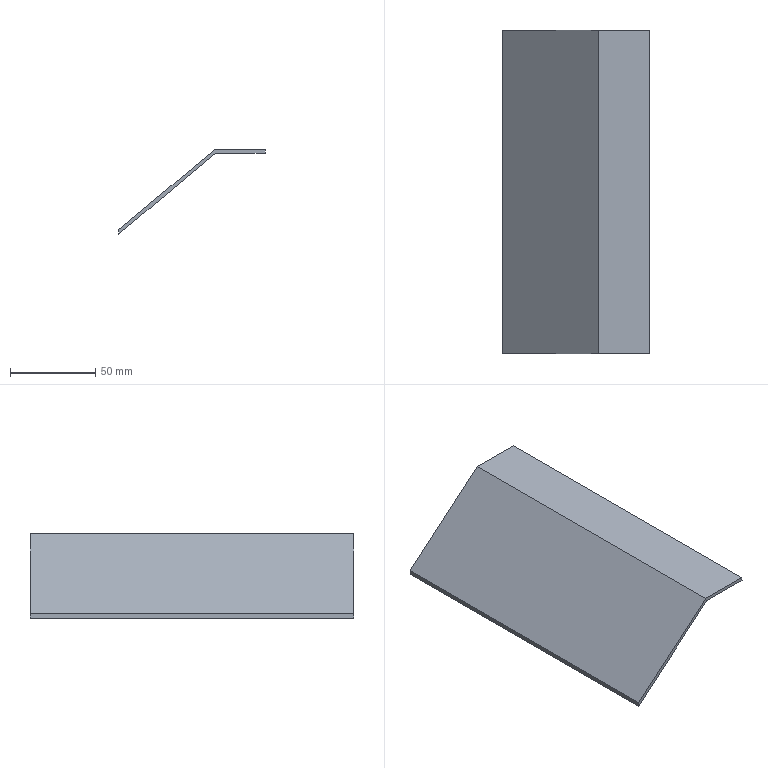Part | NX | features solid 2 | 1 solid | 8 faces | box 86 x 190 x 49.6 mm | volume 39221 mm3 | plane 8
STEP:
#1=CARTESIAN_POINT('',(-231.,-140.,-221.99));
#2=VERTEX_POINT('',#1);
#3=CARTESIAN_POINT('',(-231.,-140.,-224.6));
#4=VERTEX_POINT('',#3);
#5=CARTESIAN_POINT('',(-231.,-140.,-191.07));
#6=DIRECTION('',(0.,0.,-1.));
#7=VECTOR('',#6,1000.);
#8=LINE('',#5,#7);
#9=EDGE_CURVE('',#2,#4,#8,.T.);
#10=ORIENTED_EDGE('',*,*,#9,.F.);
#11=CARTESIAN_POINT('',(-231.,50.,-221.99));
#12=VERTEX_POINT('',#11);
#13=CARTESIAN_POINT('',(-231.,-140.,-221.99));
#14=DIRECTION('',(0.,-1.,0.));
#15=VECTOR('',#14,1000.);
#16=LINE('',#13,#15);
#17=EDGE_CURVE('',#2,#12,#16,.F.);
#18=ORIENTED_EDGE('',*,*,#17,.T.);
#19=CARTESIAN_POINT('',(-231.,50.,-224.6));
#20=VERTEX_POINT('',#19);
#21=CARTESIAN_POINT('',(-231.,50.,0.));
#22=DIRECTION('',(0.,0.,1.));
#23=VECTOR('',#22,1000.);
#24=LINE('',#21,#23);
#25=EDGE_CURVE('',#12,#20,#24,.F.);
#26=ORIENTED_EDGE('',*,*,#25,.T.);
#27=CARTESIAN_POINT('',(-231.,-140.,-224.6));
#28=DIRECTION('',(0.,-1.,0.));
#29=VECTOR('',#28,1000.);
#30=LINE('',#27,#29);
#31=EDGE_CURVE('',#4,#20,#30,.F.);
#32=ORIENTED_EDGE('',*,*,#31,.F.);
#33=EDGE_LOOP('',(#10,#18,#26,#32));
#34=FACE_BOUND('',#33,.T.);
#35=CARTESIAN_POINT('',(-231.,-400.,0.));
#36=DIRECTION('',(1.,0.,0.));
#37=DIRECTION('',(0.,0.,-1.));
#38=AXIS2_PLACEMENT_3D('',#35,#36,#37);
#39=PLANE('',#38);
#40=ADVANCED_FACE('',(#34),#39,.F.);
#41=CARTESIAN_POINT('',(-174.272,50.,-177.));
#42=VERTEX_POINT('',#41);
#43=CARTESIAN_POINT('',(-145.,50.,-177.));
#44=VERTEX_POINT('',#43);
#45=CARTESIAN_POINT('',(-175.,50.,-177.));
#46=DIRECTION('',(1.,0.,0.));
#47=VECTOR('',#46,1000.);
#48=LINE('',#45,#47);
#49=EDGE_CURVE('',#42,#44,#48,.T.);
#50=ORIENTED_EDGE('',*,*,#49,.F.);
#51=CARTESIAN_POINT('',(-192.866,50.,-192.602));
#52=DIRECTION('',(-0.766,0.,-0.6428));
#53=VECTOR('',#52,1000.);
#54=LINE('',#51,#53);
#55=EDGE_CURVE('',#20,#42,#54,.F.);
#56=ORIENTED_EDGE('',*,*,#55,.F.);
#57=ORIENTED_EDGE('',*,*,#25,.F.);
#58=CARTESIAN_POINT('',(-175.,50.,-175.));
#59=VERTEX_POINT('',#58);
#60=CARTESIAN_POINT('',(-194.151,50.,-191.07));
#61=DIRECTION('',(0.766,0.,0.6428));
#62=VECTOR('',#61,1000.);
#63=LINE('',#60,#62);
#64=EDGE_CURVE('',#12,#59,#63,.T.);
#65=ORIENTED_EDGE('',*,*,#64,.T.);
#66=CARTESIAN_POINT('',(-145.,50.,-175.));
#67=VERTEX_POINT('',#66);
#68=CARTESIAN_POINT('',(-175.,50.,-175.));
#69=DIRECTION('',(1.,0.,0.));
#70=VECTOR('',#69,1000.);
#71=LINE('',#68,#70);
#72=EDGE_CURVE('',#59,#67,#71,.T.);
#73=ORIENTED_EDGE('',*,*,#72,.T.);
#74=CARTESIAN_POINT('',(-145.,50.,-177.));
#75=DIRECTION('',(0.,0.,1.));
#76=VECTOR('',#75,1000.);
#77=LINE('',#74,#76);
#78=EDGE_CURVE('',#44,#67,#77,.T.);
#79=ORIENTED_EDGE('',*,*,#78,.F.);
#80=EDGE_LOOP('',(#50,#56,#57,#65,#73,#79));
#81=FACE_BOUND('',#80,.T.);
#82=CARTESIAN_POINT('',(-194.151,50.,-191.07));
#83=DIRECTION('',(0.,1.,0.));
#84=DIRECTION('',(0.766,0.,0.6428));
#85=AXIS2_PLACEMENT_3D('',#82,#83,#84);
#86=PLANE('',#85);
#87=ADVANCED_FACE('',(#81),#86,.T.);
#88=CARTESIAN_POINT('',(-174.272,-140.,-177.));
#89=VERTEX_POINT('',#88);
#90=CARTESIAN_POINT('',(-174.272,-140.,-177.));
#91=DIRECTION('',(0.,1.,0.));
#92=VECTOR('',#91,1000.);
#93=LINE('',#90,#92);
#94=EDGE_CURVE('',#89,#42,#93,.T.);
#95=ORIENTED_EDGE('',*,*,#94,.F.);
#96=CARTESIAN_POINT('',(-192.866,-140.,-192.602));
#97=DIRECTION('',(-0.766,0.,-0.6428));
#98=VECTOR('',#97,1000.);
#99=LINE('',#96,#98);
#100=EDGE_CURVE('',#4,#89,#99,.F.);
#101=ORIENTED_EDGE('',*,*,#100,.F.);
#102=ORIENTED_EDGE('',*,*,#31,.T.);
#103=ORIENTED_EDGE('',*,*,#55,.T.);
#104=EDGE_LOOP('',(#95,#101,#102,#103));
#105=FACE_BOUND('',#104,.T.);
#106=CARTESIAN_POINT('',(-192.866,-140.,-192.602));
#107=DIRECTION('',(0.6428,0.,-0.766));
#108=DIRECTION('',(-0.766,0.,-0.6428));
#109=AXIS2_PLACEMENT_3D('',#106,#107,#108);
#110=PLANE('',#109);
#111=ADVANCED_FACE('',(#105),#110,.T.);
#112=ORIENTED_EDGE('',*,*,#100,.T.);
#113=CARTESIAN_POINT('',(-145.,-140.,-177.));
#114=VERTEX_POINT('',#113);
#115=CARTESIAN_POINT('',(-175.,-140.,-177.));
#116=DIRECTION('',(1.,0.,0.));
#117=VECTOR('',#116,1000.);
#118=LINE('',#115,#117);
#119=EDGE_CURVE('',#89,#114,#118,.T.);
#120=ORIENTED_EDGE('',*,*,#119,.T.);
#121=CARTESIAN_POINT('',(-145.,-140.,-175.));
#122=VERTEX_POINT('',#121);
#123=CARTESIAN_POINT('',(-145.,-140.,-177.));
#124=DIRECTION('',(0.,0.,-1.));
#125=VECTOR('',#124,1000.);
#126=LINE('',#123,#125);
#127=EDGE_CURVE('',#114,#122,#126,.F.);
#128=ORIENTED_EDGE('',*,*,#127,.T.);
#129=CARTESIAN_POINT('',(-175.,-140.,-175.));
#130=VERTEX_POINT('',#129);
#131=CARTESIAN_POINT('',(-175.,-140.,-175.));
#132=DIRECTION('',(1.,0.,0.));
#133=VECTOR('',#132,1000.);
#134=LINE('',#131,#133);
#135=EDGE_CURVE('',#130,#122,#134,.T.);
#136=ORIENTED_EDGE('',*,*,#135,.F.);
#137=CARTESIAN_POINT('',(-194.151,-140.,-191.07));
#138=DIRECTION('',(0.766,0.,0.6428));
#139=VECTOR('',#138,1000.);
#140=LINE('',#137,#139);
#141=EDGE_CURVE('',#2,#130,#140,.T.);
#142=ORIENTED_EDGE('',*,*,#141,.F.);
#143=ORIENTED_EDGE('',*,*,#9,.T.);
#144=EDGE_LOOP('',(#112,#120,#128,#136,#142,#143));
#145=FACE_BOUND('',#144,.T.);
#146=CARTESIAN_POINT('',(-194.151,-140.,-191.07));
#147=DIRECTION('',(0.,1.,0.));
#148=DIRECTION('',(0.766,0.,0.6428));
#149=AXIS2_PLACEMENT_3D('',#146,#147,#148);
#150=PLANE('',#149);
#151=ADVANCED_FACE('',(#145),#150,.F.);
#152=CARTESIAN_POINT('',(-175.,277.701,-175.));
#153=DIRECTION('',(0.,-1.,0.));
#154=VECTOR('',#153,1000.);
#155=LINE('',#152,#154);
#156=EDGE_CURVE('',#130,#59,#155,.F.);
#157=ORIENTED_EDGE('',*,*,#156,.T.);
#158=ORIENTED_EDGE('',*,*,#64,.F.);
#159=ORIENTED_EDGE('',*,*,#17,.F.);
#160=ORIENTED_EDGE('',*,*,#141,.T.);
#161=EDGE_LOOP('',(#157,#158,#159,#160));
#162=FACE_BOUND('',#161,.T.);
#163=CARTESIAN_POINT('',(-194.151,-140.,-191.07));
#164=DIRECTION('',(0.6428,0.,-0.766));
#165=DIRECTION('',(-0.766,0.,-0.6428));
#166=AXIS2_PLACEMENT_3D('',#163,#164,#165);
#167=PLANE('',#166);
#168=ADVANCED_FACE('',(#162),#167,.F.);
#169=ORIENTED_EDGE('',*,*,#119,.F.);
#170=ORIENTED_EDGE('',*,*,#94,.T.);
#171=ORIENTED_EDGE('',*,*,#49,.T.);
#172=CARTESIAN_POINT('',(-145.,-140.,-177.));
#173=DIRECTION('',(0.,1.,0.));
#174=VECTOR('',#173,1000.);
#175=LINE('',#172,#174);
#176=EDGE_CURVE('',#114,#44,#175,.T.);
#177=ORIENTED_EDGE('',*,*,#176,.F.);
#178=EDGE_LOOP('',(#169,#170,#171,#177));
#179=FACE_BOUND('',#178,.T.);
#180=CARTESIAN_POINT('',(-175.,-140.,-177.));
#181=DIRECTION('',(0.,0.,-1.));
#182=DIRECTION('',(0.,1.,0.));
#183=AXIS2_PLACEMENT_3D('',#180,#181,#182);
#184=PLANE('',#183);
#185=ADVANCED_FACE('',(#179),#184,.T.);
#186=ORIENTED_EDGE('',*,*,#72,.F.);
#187=ORIENTED_EDGE('',*,*,#156,.F.);
#188=ORIENTED_EDGE('',*,*,#135,.T.);
#189=CARTESIAN_POINT('',(-145.,-140.,-175.));
#190=DIRECTION('',(0.,-1.,0.));
#191=VECTOR('',#190,1000.);
#192=LINE('',#189,#191);
#193=EDGE_CURVE('',#122,#67,#192,.F.);
#194=ORIENTED_EDGE('',*,*,#193,.T.);
#195=EDGE_LOOP('',(#186,#187,#188,#194));
#196=FACE_BOUND('',#195,.T.);
#197=CARTESIAN_POINT('',(-175.,-140.,-175.));
#198=DIRECTION('',(0.,0.,-1.));
#199=DIRECTION('',(0.,1.,0.));
#200=AXIS2_PLACEMENT_3D('',#197,#198,#199);
#201=PLANE('',#200);
#202=ADVANCED_FACE('',(#196),#201,.F.);
#203=ORIENTED_EDGE('',*,*,#193,.F.);
#204=ORIENTED_EDGE('',*,*,#127,.F.);
#205=ORIENTED_EDGE('',*,*,#176,.T.);
#206=ORIENTED_EDGE('',*,*,#78,.T.);
#207=EDGE_LOOP('',(#203,#204,#205,#206));
#208=FACE_BOUND('',#207,.T.);
#209=CARTESIAN_POINT('',(-145.,-140.,-177.));
#210=DIRECTION('',(1.,0.,0.));
#211=DIRECTION('',(0.,1.,0.));
#212=AXIS2_PLACEMENT_3D('',#209,#210,#211);
#213=PLANE('',#212);
#214=ADVANCED_FACE('',(#208),#213,.T.);
#215=CLOSED_SHELL('',(#40,#87,#111,#151,#168,#185,#202,#214));
#216=MANIFOLD_SOLID_BREP('',#215);
#217=(LENGTH_UNIT()NAMED_UNIT(*)SI_UNIT(.MILLI.,.METRE.));
#218=UNCERTAINTY_MEASURE_WITH_UNIT(LENGTH_MEASURE(0.00001),#217,'','');
#219=(NAMED_UNIT(*)PLANE_ANGLE_UNIT()SI_UNIT($,.RADIAN.));
#220=(NAMED_UNIT(*)SI_UNIT($,.STERADIAN.)SOLID_ANGLE_UNIT());
#221=(GEOMETRIC_REPRESENTATION_CONTEXT(3)GLOBAL_UNCERTAINTY_ASSIGNED_CONTEXT((#218))GLOBAL_UNIT_ASSIGNED_CONTEXT((#217,#219,#220))REPRESENTATION_CONTEXT('',''));
#222=ADVANCED_BREP_SHAPE_REPRESENTATION('',(#216),#221);